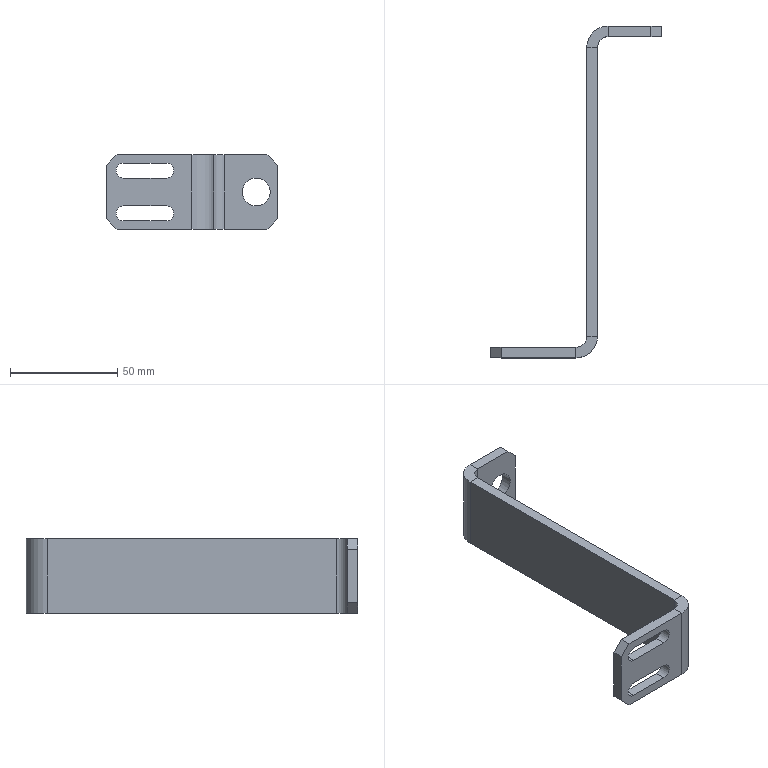Part | NX | features BREP 1 | 1 solid | 35 faces | box 80 x 155 x 35 mm | volume 36425 mm3 | plane 26 | cylinder 9 | commonest cylinder face diameters 7 x4 10 x2 20 x2 13 x1
STEP:
#1=CARTESIAN_POINT('',(0.,5.,17.5));
#2=VERTEX_POINT('',#1);
#3=CARTESIAN_POINT('',(5.,5.,17.5));
#4=VERTEX_POINT('',#3);
#5=CARTESIAN_POINT('',(0.,5.,17.5));
#6=DIRECTION('',(1.,0.,0.));
#7=VECTOR('',#6,1000.);
#8=LINE('',#5,#7);
#9=EDGE_CURVE('',#2,#4,#8,.T.);
#10=ORIENTED_EDGE('',*,*,#9,.F.);
#11=CARTESIAN_POINT('',(-5.,0.,17.5));
#12=VERTEX_POINT('',#11);
#13=CARTESIAN_POINT('',(-5.,5.,17.5));
#14=DIRECTION('',(0.,0.,1.));
#15=DIRECTION('',(-1.,0.,0.));
#16=AXIS2_PLACEMENT_3D('',#13,#14,#15);
#17=CIRCLE('',#16,5.);
#18=EDGE_CURVE('',#12,#2,#17,.T.);
#19=ORIENTED_EDGE('',*,*,#18,.F.);
#20=CARTESIAN_POINT('',(-5.,-5.,17.5));
#21=VERTEX_POINT('',#20);
#22=CARTESIAN_POINT('',(-5.,-5.,17.5));
#23=DIRECTION('',(0.,1.,0.));
#24=VECTOR('',#23,1000.);
#25=LINE('',#22,#24);
#26=EDGE_CURVE('',#21,#12,#25,.T.);
#27=ORIENTED_EDGE('',*,*,#26,.F.);
#28=CARTESIAN_POINT('',(-5.,5.,17.5));
#29=DIRECTION('',(0.,0.,1.));
#30=DIRECTION('',(1.,0.,0.));
#31=AXIS2_PLACEMENT_3D('',#28,#29,#30);
#32=CIRCLE('',#31,10.);
#33=EDGE_CURVE('',#21,#4,#32,.T.);
#34=ORIENTED_EDGE('',*,*,#33,.T.);
#35=EDGE_LOOP('',(#10,#19,#27,#34));
#36=FACE_BOUND('',#35,.T.);
#37=CARTESIAN_POINT('',(0.,5.,17.5));
#38=DIRECTION('',(0.,0.,1.));
#39=DIRECTION('',(-1.,0.,0.));
#40=AXIS2_PLACEMENT_3D('',#37,#38,#39);
#41=PLANE('',#40);
#42=ADVANCED_FACE('',(#36),#41,.T.);
#43=CARTESIAN_POINT('',(0.,140.,17.5));
#44=VERTEX_POINT('',#43);
#45=CARTESIAN_POINT('',(0.,0.,17.5));
#46=DIRECTION('',(0.,1.,0.));
#47=VECTOR('',#46,1000.);
#48=LINE('',#45,#47);
#49=EDGE_CURVE('',#2,#44,#48,.T.);
#50=ORIENTED_EDGE('',*,*,#49,.F.);
#51=ORIENTED_EDGE('',*,*,#9,.T.);
#52=CARTESIAN_POINT('',(5.,140.,17.5));
#53=VERTEX_POINT('',#52);
#54=CARTESIAN_POINT('',(5.,0.,17.5));
#55=DIRECTION('',(0.,1.,0.));
#56=VECTOR('',#55,1000.);
#57=LINE('',#54,#56);
#58=EDGE_CURVE('',#4,#53,#57,.T.);
#59=ORIENTED_EDGE('',*,*,#58,.T.);
#60=CARTESIAN_POINT('',(5.,140.,17.5));
#61=DIRECTION('',(-1.,0.,0.));
#62=VECTOR('',#61,1000.);
#63=LINE('',#60,#62);
#64=EDGE_CURVE('',#53,#44,#63,.T.);
#65=ORIENTED_EDGE('',*,*,#64,.T.);
#66=EDGE_LOOP('',(#50,#51,#59,#65));
#67=FACE_BOUND('',#66,.T.);
#68=CARTESIAN_POINT('',(-5.,-5.,17.5));
#69=DIRECTION('',(0.,0.,1.));
#70=DIRECTION('',(-1.,0.,0.));
#71=AXIS2_PLACEMENT_3D('',#68,#69,#70);
#72=PLANE('',#71);
#73=ADVANCED_FACE('',(#67),#72,.T.);
#74=CARTESIAN_POINT('',(-5.,0.,-17.5));
#75=VERTEX_POINT('',#74);
#76=CARTESIAN_POINT('',(-5.,-5.,-17.5));
#77=VERTEX_POINT('',#76);
#78=CARTESIAN_POINT('',(-5.,0.,-17.5));
#79=DIRECTION('',(0.,-1.,0.));
#80=VECTOR('',#79,1000.);
#81=LINE('',#78,#80);
#82=EDGE_CURVE('',#75,#77,#81,.T.);
#83=ORIENTED_EDGE('',*,*,#82,.F.);
#84=CARTESIAN_POINT('',(0.,5.,-17.5));
#85=VERTEX_POINT('',#84);
#86=CARTESIAN_POINT('',(-5.,5.,-17.5));
#87=DIRECTION('',(0.,0.,1.));
#88=DIRECTION('',(-1.,0.,0.));
#89=AXIS2_PLACEMENT_3D('',#86,#87,#88);
#90=CIRCLE('',#89,5.);
#91=EDGE_CURVE('',#75,#85,#90,.T.);
#92=ORIENTED_EDGE('',*,*,#91,.T.);
#93=CARTESIAN_POINT('',(5.,5.,-17.5));
#94=VERTEX_POINT('',#93);
#95=CARTESIAN_POINT('',(5.,5.,-17.5));
#96=DIRECTION('',(-1.,0.,0.));
#97=VECTOR('',#96,1000.);
#98=LINE('',#95,#97);
#99=EDGE_CURVE('',#94,#85,#98,.T.);
#100=ORIENTED_EDGE('',*,*,#99,.F.);
#101=CARTESIAN_POINT('',(-5.,5.,-17.5));
#102=DIRECTION('',(0.,0.,1.));
#103=DIRECTION('',(1.,0.,0.));
#104=AXIS2_PLACEMENT_3D('',#101,#102,#103);
#105=CIRCLE('',#104,10.);
#106=EDGE_CURVE('',#77,#94,#105,.T.);
#107=ORIENTED_EDGE('',*,*,#106,.F.);
#108=EDGE_LOOP('',(#83,#92,#100,#107));
#109=FACE_BOUND('',#108,.T.);
#110=CARTESIAN_POINT('',(-5.,0.,-17.5));
#111=DIRECTION('',(0.,0.,-1.));
#112=DIRECTION('',(1.,0.,0.));
#113=AXIS2_PLACEMENT_3D('',#110,#111,#112);
#114=PLANE('',#113);
#115=ADVANCED_FACE('',(#109),#114,.T.);
#116=CARTESIAN_POINT('',(-40.,-5.,-17.5));
#117=VERTEX_POINT('',#116);
#118=CARTESIAN_POINT('',(-45.,-5.,-17.5));
#119=DIRECTION('',(1.,0.,0.));
#120=VECTOR('',#119,1000.);
#121=LINE('',#118,#120);
#122=EDGE_CURVE('',#117,#77,#121,.T.);
#123=ORIENTED_EDGE('',*,*,#122,.F.);
#124=CARTESIAN_POINT('',(-40.,0.,-17.5));
#125=VERTEX_POINT('',#124);
#126=CARTESIAN_POINT('',(-40.,5.,-17.5));
#127=DIRECTION('',(0.,1.,0.));
#128=VECTOR('',#127,1000.);
#129=LINE('',#126,#128);
#130=EDGE_CURVE('',#117,#125,#129,.T.);
#131=ORIENTED_EDGE('',*,*,#130,.T.);
#132=CARTESIAN_POINT('',(-45.,0.,-17.5));
#133=DIRECTION('',(1.,0.,0.));
#134=VECTOR('',#133,1000.);
#135=LINE('',#132,#134);
#136=EDGE_CURVE('',#125,#75,#135,.T.);
#137=ORIENTED_EDGE('',*,*,#136,.T.);
#138=ORIENTED_EDGE('',*,*,#82,.T.);
#139=EDGE_LOOP('',(#123,#131,#137,#138));
#140=FACE_BOUND('',#139,.T.);
#141=CARTESIAN_POINT('',(5.,5.,-17.5));
#142=DIRECTION('',(0.,0.,-1.));
#143=DIRECTION('',(1.,0.,0.));
#144=AXIS2_PLACEMENT_3D('',#141,#142,#143);
#145=PLANE('',#144);
#146=ADVANCED_FACE('',(#140),#145,.T.);
#147=CARTESIAN_POINT('',(10.,150.,17.5));
#148=VERTEX_POINT('',#147);
#149=CARTESIAN_POINT('',(10.,145.,17.5));
#150=VERTEX_POINT('',#149);
#151=CARTESIAN_POINT('',(10.,150.,17.5));
#152=DIRECTION('',(0.,-1.,0.));
#153=VECTOR('',#152,1000.);
#154=LINE('',#151,#153);
#155=EDGE_CURVE('',#148,#150,#154,.T.);
#156=ORIENTED_EDGE('',*,*,#155,.F.);
#157=CARTESIAN_POINT('',(10.,140.,17.5));
#158=DIRECTION('',(0.,0.,-1.));
#159=DIRECTION('',(1.,0.,0.));
#160=AXIS2_PLACEMENT_3D('',#157,#158,#159);
#161=CIRCLE('',#160,10.);
#162=EDGE_CURVE('',#44,#148,#161,.T.);
#163=ORIENTED_EDGE('',*,*,#162,.F.);
#164=ORIENTED_EDGE('',*,*,#64,.F.);
#165=CARTESIAN_POINT('',(10.,140.,17.5));
#166=DIRECTION('',(0.,0.,-1.));
#167=DIRECTION('',(1.,0.,0.));
#168=AXIS2_PLACEMENT_3D('',#165,#166,#167);
#169=CIRCLE('',#168,5.);
#170=EDGE_CURVE('',#53,#150,#169,.T.);
#171=ORIENTED_EDGE('',*,*,#170,.T.);
#172=EDGE_LOOP('',(#156,#163,#164,#171));
#173=FACE_BOUND('',#172,.T.);
#174=CARTESIAN_POINT('',(10.,150.,17.5));
#175=DIRECTION('',(0.,0.,1.));
#176=DIRECTION('',(-1.,0.,0.));
#177=AXIS2_PLACEMENT_3D('',#174,#175,#176);
#178=PLANE('',#177);
#179=ADVANCED_FACE('',(#173),#178,.T.);
#180=CARTESIAN_POINT('',(30.,145.,17.5));
#181=VERTEX_POINT('',#180);
#182=CARTESIAN_POINT('',(0.,145.,17.5));
#183=DIRECTION('',(1.,0.,0.));
#184=VECTOR('',#183,1000.);
#185=LINE('',#182,#184);
#186=EDGE_CURVE('',#150,#181,#185,.T.);
#187=ORIENTED_EDGE('',*,*,#186,.T.);
#188=CARTESIAN_POINT('',(30.,150.,17.5));
#189=VERTEX_POINT('',#188);
#190=CARTESIAN_POINT('',(30.,140.,17.5));
#191=DIRECTION('',(0.,1.,0.));
#192=VECTOR('',#191,1000.);
#193=LINE('',#190,#192);
#194=EDGE_CURVE('',#181,#189,#193,.T.);
#195=ORIENTED_EDGE('',*,*,#194,.T.);
#196=CARTESIAN_POINT('',(0.,150.,17.5));
#197=DIRECTION('',(1.,0.,0.));
#198=VECTOR('',#197,1000.);
#199=LINE('',#196,#198);
#200=EDGE_CURVE('',#148,#189,#199,.T.);
#201=ORIENTED_EDGE('',*,*,#200,.F.);
#202=ORIENTED_EDGE('',*,*,#155,.T.);
#203=EDGE_LOOP('',(#187,#195,#201,#202));
#204=FACE_BOUND('',#203,.T.);
#205=CARTESIAN_POINT('',(5.,140.,17.5));
#206=DIRECTION('',(0.,0.,1.));
#207=DIRECTION('',(-1.,0.,0.));
#208=AXIS2_PLACEMENT_3D('',#205,#206,#207);
#209=PLANE('',#208);
#210=ADVANCED_FACE('',(#204),#209,.T.);
#211=CARTESIAN_POINT('',(0.,140.,-17.5));
#212=VERTEX_POINT('',#211);
#213=CARTESIAN_POINT('',(5.,140.,-17.5));
#214=VERTEX_POINT('',#213);
#215=CARTESIAN_POINT('',(0.,140.,-17.5));
#216=DIRECTION('',(1.,0.,0.));
#217=VECTOR('',#216,1000.);
#218=LINE('',#215,#217);
#219=EDGE_CURVE('',#212,#214,#218,.T.);
#220=ORIENTED_EDGE('',*,*,#219,.F.);
#221=CARTESIAN_POINT('',(10.,150.,-17.5));
#222=VERTEX_POINT('',#221);
#223=CARTESIAN_POINT('',(10.,140.,-17.5));
#224=DIRECTION('',(0.,0.,-1.));
#225=DIRECTION('',(1.,0.,0.));
#226=AXIS2_PLACEMENT_3D('',#223,#224,#225);
#227=CIRCLE('',#226,10.);
#228=EDGE_CURVE('',#212,#222,#227,.T.);
#229=ORIENTED_EDGE('',*,*,#228,.T.);
#230=CARTESIAN_POINT('',(10.,145.,-17.5));
#231=VERTEX_POINT('',#230);
#232=CARTESIAN_POINT('',(10.,145.,-17.5));
#233=DIRECTION('',(0.,1.,0.));
#234=VECTOR('',#233,1000.);
#235=LINE('',#232,#234);
#236=EDGE_CURVE('',#231,#222,#235,.T.);
#237=ORIENTED_EDGE('',*,*,#236,.F.);
#238=CARTESIAN_POINT('',(10.,140.,-17.5));
#239=DIRECTION('',(0.,0.,-1.));
#240=DIRECTION('',(1.,0.,0.));
#241=AXIS2_PLACEMENT_3D('',#238,#239,#240);
#242=CIRCLE('',#241,5.);
#243=EDGE_CURVE('',#214,#231,#242,.T.);
#244=ORIENTED_EDGE('',*,*,#243,.F.);
#245=EDGE_LOOP('',(#220,#229,#237,#244));
#246=FACE_BOUND('',#245,.T.);
#247=CARTESIAN_POINT('',(0.,140.,-17.5));
#248=DIRECTION('',(0.,0.,-1.));
#249=DIRECTION('',(1.,0.,0.));
#250=AXIS2_PLACEMENT_3D('',#247,#248,#249);
#251=PLANE('',#250);
#252=ADVANCED_FACE('',(#246),#251,.T.);
#253=CARTESIAN_POINT('',(0.,0.,-17.5));
#254=DIRECTION('',(0.,1.,0.));
#255=VECTOR('',#254,1000.);
#256=LINE('',#253,#255);
#257=EDGE_CURVE('',#85,#212,#256,.T.);
#258=ORIENTED_EDGE('',*,*,#257,.T.);
#259=ORIENTED_EDGE('',*,*,#219,.T.);
#260=CARTESIAN_POINT('',(5.,0.,-17.5));
#261=DIRECTION('',(0.,1.,0.));
#262=VECTOR('',#261,1000.);
#263=LINE('',#260,#262);
#264=EDGE_CURVE('',#94,#214,#263,.T.);
#265=ORIENTED_EDGE('',*,*,#264,.F.);
#266=ORIENTED_EDGE('',*,*,#99,.T.);
#267=EDGE_LOOP('',(#258,#259,#265,#266));
#268=FACE_BOUND('',#267,.T.);
#269=CARTESIAN_POINT('',(10.,145.,-17.5));
#270=DIRECTION('',(0.,0.,-1.));
#271=DIRECTION('',(1.,0.,0.));
#272=AXIS2_PLACEMENT_3D('',#269,#270,#271);
#273=PLANE('',#272);
#274=ADVANCED_FACE('',(#268),#273,.T.);
#275=CARTESIAN_POINT('',(25.,145.,6.5));
#276=VERTEX_POINT('',#275);
#277=CARTESIAN_POINT('',(25.,145.,0.));
#278=DIRECTION('',(0.,1.,0.));
#279=DIRECTION('',(0.,0.,1.));
#280=AXIS2_PLACEMENT_3D('',#277,#278,#279);
#281=CIRCLE('',#280,6.5);
#282=EDGE_CURVE('',#276,#276,#281,.T.);
#283=ORIENTED_EDGE('',*,*,#282,.T.);
#284=EDGE_LOOP('',(#283));
#285=FACE_BOUND('',#284,.T.);
#286=CARTESIAN_POINT('',(35.,145.,12.5));
#287=VERTEX_POINT('',#286);
#288=CARTESIAN_POINT('',(35.,145.,-12.5));
#289=VERTEX_POINT('',#288);
#290=CARTESIAN_POINT('',(35.,145.,17.5));
#291=DIRECTION('',(0.,0.,-1.));
#292=VECTOR('',#291,1000.);
#293=LINE('',#290,#292);
#294=EDGE_CURVE('',#287,#289,#293,.T.);
#295=ORIENTED_EDGE('',*,*,#294,.F.);
#296=CARTESIAN_POINT('',(35.,145.,12.5));
#297=DIRECTION('',(-0.7071,0.,0.7071));
#298=VECTOR('',#297,1000.);
#299=LINE('',#296,#298);
#300=EDGE_CURVE('',#287,#181,#299,.T.);
#301=ORIENTED_EDGE('',*,*,#300,.T.);
#302=ORIENTED_EDGE('',*,*,#186,.F.);
#303=CARTESIAN_POINT('',(10.,145.,17.5));
#304=DIRECTION('',(0.,0.,-1.));
#305=VECTOR('',#304,1000.);
#306=LINE('',#303,#305);
#307=EDGE_CURVE('',#150,#231,#306,.T.);
#308=ORIENTED_EDGE('',*,*,#307,.T.);
#309=CARTESIAN_POINT('',(30.,145.,-17.5));
#310=VERTEX_POINT('',#309);
#311=CARTESIAN_POINT('',(0.,145.,-17.5));
#312=DIRECTION('',(1.,0.,0.));
#313=VECTOR('',#312,1000.);
#314=LINE('',#311,#313);
#315=EDGE_CURVE('',#231,#310,#314,.T.);
#316=ORIENTED_EDGE('',*,*,#315,.T.);
#317=CARTESIAN_POINT('',(30.,145.,-17.5));
#318=DIRECTION('',(0.7071,0.,0.7071));
#319=VECTOR('',#318,1000.);
#320=LINE('',#317,#319);
#321=EDGE_CURVE('',#310,#289,#320,.T.);
#322=ORIENTED_EDGE('',*,*,#321,.T.);
#323=EDGE_LOOP('',(#295,#301,#302,#308,#316,#322));
#324=FACE_BOUND('',#323,.T.);
#325=CARTESIAN_POINT('',(0.,145.,17.5));
#326=DIRECTION('',(0.,1.,0.));
#327=DIRECTION('',(0.,0.,-1.));
#328=AXIS2_PLACEMENT_3D('',#325,#326,#327);
#329=PLANE('',#328);
#330=ADVANCED_FACE('',(#285,#324),#329,.F.);
#331=CARTESIAN_POINT('',(35.,150.,12.5));
#332=VERTEX_POINT('',#331);
#333=CARTESIAN_POINT('',(35.,150.,-12.5));
#334=VERTEX_POINT('',#333);
#335=CARTESIAN_POINT('',(35.,150.,17.5));
#336=DIRECTION('',(0.,0.,-1.));
#337=VECTOR('',#336,1000.);
#338=LINE('',#335,#337);
#339=EDGE_CURVE('',#332,#334,#338,.T.);
#340=ORIENTED_EDGE('',*,*,#339,.F.);
#341=CARTESIAN_POINT('',(35.,150.,12.5));
#342=DIRECTION('',(0.,-1.,0.));
#343=VECTOR('',#342,1000.);
#344=LINE('',#341,#343);
#345=EDGE_CURVE('',#332,#287,#344,.T.);
#346=ORIENTED_EDGE('',*,*,#345,.T.);
#347=ORIENTED_EDGE('',*,*,#294,.T.);
#348=CARTESIAN_POINT('',(35.,150.,-12.5));
#349=DIRECTION('',(0.,1.,0.));
#350=VECTOR('',#349,1000.);
#351=LINE('',#348,#350);
#352=EDGE_CURVE('',#289,#334,#351,.T.);
#353=ORIENTED_EDGE('',*,*,#352,.T.);
#354=EDGE_LOOP('',(#340,#346,#347,#353));
#355=FACE_BOUND('',#354,.T.);
#356=CARTESIAN_POINT('',(35.,150.,17.5));
#357=DIRECTION('',(1.,0.,0.));
#358=DIRECTION('',(0.,0.,1.));
#359=AXIS2_PLACEMENT_3D('',#356,#357,#358);
#360=PLANE('',#359);
#361=ADVANCED_FACE('',(#355),#360,.T.);
#362=CARTESIAN_POINT('',(25.,150.,6.5));
#363=VERTEX_POINT('',#362);
#364=CARTESIAN_POINT('',(25.,150.,0.));
#365=DIRECTION('',(0.,1.,0.));
#366=DIRECTION('',(0.,0.,1.));
#367=AXIS2_PLACEMENT_3D('',#364,#365,#366);
#368=CIRCLE('',#367,6.5);
#369=EDGE_CURVE('',#363,#363,#368,.T.);
#370=ORIENTED_EDGE('',*,*,#369,.F.);
#371=EDGE_LOOP('',(#370));
#372=FACE_BOUND('',#371,.T.);
#373=ORIENTED_EDGE('',*,*,#200,.T.);
#374=CARTESIAN_POINT('',(15.,150.,32.5));
#375=DIRECTION('',(0.7071,0.,-0.7071));
#376=VECTOR('',#375,1000.);
#377=LINE('',#374,#376);
#378=EDGE_CURVE('',#189,#332,#377,.T.);
#379=ORIENTED_EDGE('',*,*,#378,.T.);
#380=ORIENTED_EDGE('',*,*,#339,.T.);
#381=CARTESIAN_POINT('',(30.,150.,-17.5));
#382=VERTEX_POINT('',#381);
#383=CARTESIAN_POINT('',(32.5,150.,-15.));
#384=DIRECTION('',(-0.7071,0.,-0.7071));
#385=VECTOR('',#384,1000.);
#386=LINE('',#383,#385);
#387=EDGE_CURVE('',#334,#382,#386,.T.);
#388=ORIENTED_EDGE('',*,*,#387,.T.);
#389=CARTESIAN_POINT('',(0.,150.,-17.5));
#390=DIRECTION('',(1.,0.,0.));
#391=VECTOR('',#390,1000.);
#392=LINE('',#389,#391);
#393=EDGE_CURVE('',#222,#382,#392,.T.);
#394=ORIENTED_EDGE('',*,*,#393,.F.);
#395=CARTESIAN_POINT('',(10.,150.,17.5));
#396=DIRECTION('',(0.,0.,-1.));
#397=VECTOR('',#396,1000.);
#398=LINE('',#395,#397);
#399=EDGE_CURVE('',#148,#222,#398,.T.);
#400=ORIENTED_EDGE('',*,*,#399,.F.);
#401=EDGE_LOOP('',(#373,#379,#380,#388,#394,#400));
#402=FACE_BOUND('',#401,.T.);
#403=CARTESIAN_POINT('',(0.,150.,17.5));
#404=DIRECTION('',(0.,1.,0.));
#405=DIRECTION('',(0.,0.,-1.));
#406=AXIS2_PLACEMENT_3D('',#403,#404,#405);
#407=PLANE('',#406);
#408=ADVANCED_FACE('',(#372,#402),#407,.T.);
#409=ORIENTED_EDGE('',*,*,#228,.F.);
#410=CARTESIAN_POINT('',(0.,140.,17.5));
#411=DIRECTION('',(0.,0.,-1.));
#412=VECTOR('',#411,1000.);
#413=LINE('',#410,#412);
#414=EDGE_CURVE('',#44,#212,#413,.T.);
#415=ORIENTED_EDGE('',*,*,#414,.F.);
#416=ORIENTED_EDGE('',*,*,#162,.T.);
#417=ORIENTED_EDGE('',*,*,#399,.T.);
#418=EDGE_LOOP('',(#409,#415,#416,#417));
#419=FACE_BOUND('',#418,.T.);
#420=CARTESIAN_POINT('',(10.,140.,17.5));
#421=DIRECTION('',(0.,0.,-1.));
#422=DIRECTION('',(1.,0.,0.));
#423=AXIS2_PLACEMENT_3D('',#420,#421,#422);
#424=CYLINDRICAL_SURFACE('',#423,10.);
#425=ADVANCED_FACE('',(#419),#424,.T.);
#426=ORIENTED_EDGE('',*,*,#257,.F.);
#427=CARTESIAN_POINT('',(0.,5.,17.5));
#428=DIRECTION('',(0.,0.,-1.));
#429=VECTOR('',#428,1000.);
#430=LINE('',#427,#429);
#431=EDGE_CURVE('',#2,#85,#430,.T.);
#432=ORIENTED_EDGE('',*,*,#431,.F.);
#433=ORIENTED_EDGE('',*,*,#49,.T.);
#434=ORIENTED_EDGE('',*,*,#414,.T.);
#435=EDGE_LOOP('',(#426,#432,#433,#434));
#436=FACE_BOUND('',#435,.T.);
#437=CARTESIAN_POINT('',(0.,0.,17.5));
#438=DIRECTION('',(-1.,0.,0.));
#439=DIRECTION('',(0.,0.,-1.));
#440=AXIS2_PLACEMENT_3D('',#437,#438,#439);
#441=PLANE('',#440);
#442=ADVANCED_FACE('',(#436),#441,.T.);
#443=ORIENTED_EDGE('',*,*,#91,.F.);
#444=CARTESIAN_POINT('',(-5.,0.,17.5));
#445=DIRECTION('',(0.,0.,-1.));
#446=VECTOR('',#445,1000.);
#447=LINE('',#444,#446);
#448=EDGE_CURVE('',#12,#75,#447,.T.);
#449=ORIENTED_EDGE('',*,*,#448,.F.);
#450=ORIENTED_EDGE('',*,*,#18,.T.);
#451=ORIENTED_EDGE('',*,*,#431,.T.);
#452=EDGE_LOOP('',(#443,#449,#450,#451));
#453=FACE_BOUND('',#452,.T.);
#454=CARTESIAN_POINT('',(-5.,5.,17.5));
#455=DIRECTION('',(0.,0.,-1.));
#456=DIRECTION('',(1.,0.,0.));
#457=AXIS2_PLACEMENT_3D('',#454,#455,#456);
#458=CYLINDRICAL_SURFACE('',#457,5.);
#459=ADVANCED_FACE('',(#453),#458,.F.);
#460=CARTESIAN_POINT('',(-37.,0.,-13.5));
#461=VERTEX_POINT('',#460);
#462=CARTESIAN_POINT('',(-17.,0.,-13.5));
#463=VERTEX_POINT('',#462);
#464=CARTESIAN_POINT('',(-37.,0.,-13.5));
#465=DIRECTION('',(1.,0.,0.));
#466=VECTOR('',#465,1000.);
#467=LINE('',#464,#466);
#468=EDGE_CURVE('',#461,#463,#467,.T.);
#469=ORIENTED_EDGE('',*,*,#468,.T.);
#470=CARTESIAN_POINT('',(-17.,0.,-6.5));
#471=VERTEX_POINT('',#470);
#472=CARTESIAN_POINT('',(-17.,0.,-10.));
#473=DIRECTION('',(0.,-1.,0.));
#474=DIRECTION('',(0.,0.,1.));
#475=AXIS2_PLACEMENT_3D('',#472,#473,#474);
#476=CIRCLE('',#475,3.5);
#477=EDGE_CURVE('',#463,#471,#476,.T.);
#478=ORIENTED_EDGE('',*,*,#477,.T.);
#479=CARTESIAN_POINT('',(-37.,0.,-6.5));
#480=VERTEX_POINT('',#479);
#481=CARTESIAN_POINT('',(-37.,0.,-6.5));
#482=DIRECTION('',(-1.,0.,0.));
#483=VECTOR('',#482,1000.);
#484=LINE('',#481,#483);
#485=EDGE_CURVE('',#471,#480,#484,.T.);
#486=ORIENTED_EDGE('',*,*,#485,.T.);
#487=CARTESIAN_POINT('',(-37.,0.,-10.));
#488=DIRECTION('',(0.,-1.,0.));
#489=DIRECTION('',(0.,0.,1.));
#490=AXIS2_PLACEMENT_3D('',#487,#488,#489);
#491=CIRCLE('',#490,3.5);
#492=EDGE_CURVE('',#480,#461,#491,.T.);
#493=ORIENTED_EDGE('',*,*,#492,.T.);
#494=EDGE_LOOP('',(#469,#478,#486,#493));
#495=FACE_BOUND('',#494,.T.);
#496=CARTESIAN_POINT('',(-37.,0.,6.5));
#497=VERTEX_POINT('',#496);
#498=CARTESIAN_POINT('',(-17.,0.,6.5));
#499=VERTEX_POINT('',#498);
#500=CARTESIAN_POINT('',(-37.,0.,6.5));
#501=DIRECTION('',(1.,0.,0.));
#502=VECTOR('',#501,1000.);
#503=LINE('',#500,#502);
#504=EDGE_CURVE('',#497,#499,#503,.T.);
#505=ORIENTED_EDGE('',*,*,#504,.T.);
#506=CARTESIAN_POINT('',(-17.,0.,13.5));
#507=VERTEX_POINT('',#506);
#508=CARTESIAN_POINT('',(-17.,0.,10.));
#509=DIRECTION('',(0.,-1.,0.));
#510=DIRECTION('',(0.,0.,1.));
#511=AXIS2_PLACEMENT_3D('',#508,#509,#510);
#512=CIRCLE('',#511,3.5);
#513=EDGE_CURVE('',#499,#507,#512,.T.);
#514=ORIENTED_EDGE('',*,*,#513,.T.);
#515=CARTESIAN_POINT('',(-37.,0.,13.5));
#516=VERTEX_POINT('',#515);
#517=CARTESIAN_POINT('',(-37.,0.,13.5));
#518=DIRECTION('',(-1.,0.,0.));
#519=VECTOR('',#518,1000.);
#520=LINE('',#517,#519);
#521=EDGE_CURVE('',#507,#516,#520,.T.);
#522=ORIENTED_EDGE('',*,*,#521,.T.);
#523=CARTESIAN_POINT('',(-37.,0.,10.));
#524=DIRECTION('',(0.,-1.,0.));
#525=DIRECTION('',(0.,0.,1.));
#526=AXIS2_PLACEMENT_3D('',#523,#524,#525);
#527=CIRCLE('',#526,3.5);
#528=EDGE_CURVE('',#516,#497,#527,.T.);
#529=ORIENTED_EDGE('',*,*,#528,.T.);
#530=EDGE_LOOP('',(#505,#514,#522,#529));
#531=FACE_BOUND('',#530,.T.);
#532=CARTESIAN_POINT('',(-45.,0.,12.5));
#533=VERTEX_POINT('',#532);
#534=CARTESIAN_POINT('',(-45.,0.,-12.5));
#535=VERTEX_POINT('',#534);
#536=CARTESIAN_POINT('',(-45.,0.,17.5));
#537=DIRECTION('',(0.,0.,-1.));
#538=VECTOR('',#537,1000.);
#539=LINE('',#536,#538);
#540=EDGE_CURVE('',#533,#535,#539,.T.);
#541=ORIENTED_EDGE('',*,*,#540,.F.);
#542=CARTESIAN_POINT('',(-40.,0.,17.5));
#543=VERTEX_POINT('',#542);
#544=CARTESIAN_POINT('',(-42.5,0.,15.));
#545=DIRECTION('',(0.7071,0.,0.7071));
#546=VECTOR('',#545,1000.);
#547=LINE('',#544,#546);
#548=EDGE_CURVE('',#533,#543,#547,.T.);
#549=ORIENTED_EDGE('',*,*,#548,.T.);
#550=CARTESIAN_POINT('',(-45.,0.,17.5));
#551=DIRECTION('',(1.,0.,0.));
#552=VECTOR('',#551,1000.);
#553=LINE('',#550,#552);
#554=EDGE_CURVE('',#543,#12,#553,.T.);
#555=ORIENTED_EDGE('',*,*,#554,.T.);
#556=ORIENTED_EDGE('',*,*,#448,.T.);
#557=ORIENTED_EDGE('',*,*,#136,.F.);
#558=CARTESIAN_POINT('',(-60.,0.,2.5));
#559=DIRECTION('',(-0.7071,0.,0.7071));
#560=VECTOR('',#559,1000.);
#561=LINE('',#558,#560);
#562=EDGE_CURVE('',#125,#535,#561,.T.);
#563=ORIENTED_EDGE('',*,*,#562,.T.);
#564=EDGE_LOOP('',(#541,#549,#555,#556,#557,#563));
#565=FACE_BOUND('',#564,.T.);
#566=CARTESIAN_POINT('',(-45.,0.,17.5));
#567=DIRECTION('',(0.,1.,0.));
#568=DIRECTION('',(0.,0.,-1.));
#569=AXIS2_PLACEMENT_3D('',#566,#567,#568);
#570=PLANE('',#569);
#571=ADVANCED_FACE('',(#495,#531,#565),#570,.T.);
#572=CARTESIAN_POINT('',(-45.,-5.,12.5));
#573=VERTEX_POINT('',#572);
#574=CARTESIAN_POINT('',(-45.,-5.,-12.5));
#575=VERTEX_POINT('',#574);
#576=CARTESIAN_POINT('',(-45.,-5.,17.5));
#577=DIRECTION('',(0.,0.,-1.));
#578=VECTOR('',#577,1000.);
#579=LINE('',#576,#578);
#580=EDGE_CURVE('',#573,#575,#579,.T.);
#581=ORIENTED_EDGE('',*,*,#580,.F.);
#582=CARTESIAN_POINT('',(-45.,-5.,12.5));
#583=DIRECTION('',(0.,1.,0.));
#584=VECTOR('',#583,1000.);
#585=LINE('',#582,#584);
#586=EDGE_CURVE('',#573,#533,#585,.T.);
#587=ORIENTED_EDGE('',*,*,#586,.T.);
#588=ORIENTED_EDGE('',*,*,#540,.T.);
#589=CARTESIAN_POINT('',(-45.,-5.,-12.5));
#590=DIRECTION('',(0.,-1.,0.));
#591=VECTOR('',#590,1000.);
#592=LINE('',#589,#591);
#593=EDGE_CURVE('',#535,#575,#592,.T.);
#594=ORIENTED_EDGE('',*,*,#593,.T.);
#595=EDGE_LOOP('',(#581,#587,#588,#594));
#596=FACE_BOUND('',#595,.T.);
#597=CARTESIAN_POINT('',(-45.,-5.,17.5));
#598=DIRECTION('',(-1.,0.,0.));
#599=DIRECTION('',(0.,0.,-1.));
#600=AXIS2_PLACEMENT_3D('',#597,#598,#599);
#601=PLANE('',#600);
#602=ADVANCED_FACE('',(#596),#601,.T.);
#603=CARTESIAN_POINT('',(-17.,-5.,-13.5));
#604=VERTEX_POINT('',#603);
#605=CARTESIAN_POINT('',(-17.,-5.,-6.5));
#606=VERTEX_POINT('',#605);
#607=CARTESIAN_POINT('',(-17.,-5.,-10.));
#608=DIRECTION('',(0.,-1.,0.));
#609=DIRECTION('',(1.,0.,0.));
#610=AXIS2_PLACEMENT_3D('',#607,#608,#609);
#611=CIRCLE('',#610,3.5);
#612=EDGE_CURVE('',#604,#606,#611,.T.);
#613=ORIENTED_EDGE('',*,*,#612,.F.);
#614=CARTESIAN_POINT('',(-37.,-5.,-13.5));
#615=VERTEX_POINT('',#614);
#616=CARTESIAN_POINT('',(-37.,-5.,-13.5));
#617=DIRECTION('',(1.,0.,0.));
#618=VECTOR('',#617,1000.);
#619=LINE('',#616,#618);
#620=EDGE_CURVE('',#615,#604,#619,.T.);
#621=ORIENTED_EDGE('',*,*,#620,.F.);
#622=CARTESIAN_POINT('',(-37.,-5.,-6.5));
#623=VERTEX_POINT('',#622);
#624=CARTESIAN_POINT('',(-37.,-5.,-10.));
#625=DIRECTION('',(0.,-1.,0.));
#626=DIRECTION('',(1.,0.,0.));
#627=AXIS2_PLACEMENT_3D('',#624,#625,#626);
#628=CIRCLE('',#627,3.5);
#629=EDGE_CURVE('',#623,#615,#628,.T.);
#630=ORIENTED_EDGE('',*,*,#629,.F.);
#631=CARTESIAN_POINT('',(-37.,-5.,-6.5));
#632=DIRECTION('',(-1.,0.,0.));
#633=VECTOR('',#632,1000.);
#634=LINE('',#631,#633);
#635=EDGE_CURVE('',#606,#623,#634,.T.);
#636=ORIENTED_EDGE('',*,*,#635,.F.);
#637=EDGE_LOOP('',(#613,#621,#630,#636));
#638=FACE_BOUND('',#637,.T.);
#639=CARTESIAN_POINT('',(-17.,-5.,6.5));
#640=VERTEX_POINT('',#639);
#641=CARTESIAN_POINT('',(-17.,-5.,13.5));
#642=VERTEX_POINT('',#641);
#643=CARTESIAN_POINT('',(-17.,-5.,10.));
#644=DIRECTION('',(0.,-1.,0.));
#645=DIRECTION('',(1.,0.,0.));
#646=AXIS2_PLACEMENT_3D('',#643,#644,#645);
#647=CIRCLE('',#646,3.5);
#648=EDGE_CURVE('',#640,#642,#647,.T.);
#649=ORIENTED_EDGE('',*,*,#648,.F.);
#650=CARTESIAN_POINT('',(-37.,-5.,6.5));
#651=VERTEX_POINT('',#650);
#652=CARTESIAN_POINT('',(-37.,-5.,6.5));
#653=DIRECTION('',(1.,0.,0.));
#654=VECTOR('',#653,1000.);
#655=LINE('',#652,#654);
#656=EDGE_CURVE('',#651,#640,#655,.T.);
#657=ORIENTED_EDGE('',*,*,#656,.F.);
#658=CARTESIAN_POINT('',(-37.,-5.,13.5));
#659=VERTEX_POINT('',#658);
#660=CARTESIAN_POINT('',(-37.,-5.,10.));
#661=DIRECTION('',(0.,-1.,0.));
#662=DIRECTION('',(1.,0.,0.));
#663=AXIS2_PLACEMENT_3D('',#660,#661,#662);
#664=CIRCLE('',#663,3.5);
#665=EDGE_CURVE('',#659,#651,#664,.T.);
#666=ORIENTED_EDGE('',*,*,#665,.F.);
#667=CARTESIAN_POINT('',(-37.,-5.,13.5));
#668=DIRECTION('',(-1.,0.,0.));
#669=VECTOR('',#668,1000.);
#670=LINE('',#667,#669);
#671=EDGE_CURVE('',#642,#659,#670,.T.);
#672=ORIENTED_EDGE('',*,*,#671,.F.);
#673=EDGE_LOOP('',(#649,#657,#666,#672));
#674=FACE_BOUND('',#673,.T.);
#675=CARTESIAN_POINT('',(-40.,-5.,17.5));
#676=VERTEX_POINT('',#675);
#677=CARTESIAN_POINT('',(-45.,-5.,17.5));
#678=DIRECTION('',(1.,0.,0.));
#679=VECTOR('',#678,1000.);
#680=LINE('',#677,#679);
#681=EDGE_CURVE('',#676,#21,#680,.T.);
#682=ORIENTED_EDGE('',*,*,#681,.F.);
#683=CARTESIAN_POINT('',(-45.,-5.,12.5));
#684=DIRECTION('',(-0.7071,0.,-0.7071));
#685=VECTOR('',#684,1000.);
#686=LINE('',#683,#685);
#687=EDGE_CURVE('',#676,#573,#686,.T.);
#688=ORIENTED_EDGE('',*,*,#687,.T.);
#689=ORIENTED_EDGE('',*,*,#580,.T.);
#690=CARTESIAN_POINT('',(-40.,-5.,-17.5));
#691=DIRECTION('',(0.7071,0.,-0.7071));
#692=VECTOR('',#691,1000.);
#693=LINE('',#690,#692);
#694=EDGE_CURVE('',#575,#117,#693,.T.);
#695=ORIENTED_EDGE('',*,*,#694,.T.);
#696=ORIENTED_EDGE('',*,*,#122,.T.);
#697=CARTESIAN_POINT('',(-5.,-5.,17.5));
#698=DIRECTION('',(0.,0.,-1.));
#699=VECTOR('',#698,1000.);
#700=LINE('',#697,#699);
#701=EDGE_CURVE('',#21,#77,#700,.T.);
#702=ORIENTED_EDGE('',*,*,#701,.F.);
#703=EDGE_LOOP('',(#682,#688,#689,#695,#696,#702));
#704=FACE_BOUND('',#703,.T.);
#705=CARTESIAN_POINT('',(-45.,-5.,17.5));
#706=DIRECTION('',(0.,1.,0.));
#707=DIRECTION('',(0.,0.,-1.));
#708=AXIS2_PLACEMENT_3D('',#705,#706,#707);
#709=PLANE('',#708);
#710=ADVANCED_FACE('',(#638,#674,#704),#709,.F.);
#711=ORIENTED_EDGE('',*,*,#106,.T.);
#712=CARTESIAN_POINT('',(5.,5.,17.5));
#713=DIRECTION('',(0.,0.,-1.));
#714=VECTOR('',#713,1000.);
#715=LINE('',#712,#714);
#716=EDGE_CURVE('',#4,#94,#715,.T.);
#717=ORIENTED_EDGE('',*,*,#716,.F.);
#718=ORIENTED_EDGE('',*,*,#33,.F.);
#719=ORIENTED_EDGE('',*,*,#701,.T.);
#720=EDGE_LOOP('',(#711,#717,#718,#719));
#721=FACE_BOUND('',#720,.T.);
#722=CARTESIAN_POINT('',(-5.,5.,17.5));
#723=DIRECTION('',(0.,0.,-1.));
#724=DIRECTION('',(1.,0.,0.));
#725=AXIS2_PLACEMENT_3D('',#722,#723,#724);
#726=CYLINDRICAL_SURFACE('',#725,10.);
#727=ADVANCED_FACE('',(#721),#726,.T.);
#728=ORIENTED_EDGE('',*,*,#264,.T.);
#729=CARTESIAN_POINT('',(5.,140.,17.5));
#730=DIRECTION('',(0.,0.,-1.));
#731=VECTOR('',#730,1000.);
#732=LINE('',#729,#731);
#733=EDGE_CURVE('',#53,#214,#732,.T.);
#734=ORIENTED_EDGE('',*,*,#733,.F.);
#735=ORIENTED_EDGE('',*,*,#58,.F.);
#736=ORIENTED_EDGE('',*,*,#716,.T.);
#737=EDGE_LOOP('',(#728,#734,#735,#736));
#738=FACE_BOUND('',#737,.T.);
#739=CARTESIAN_POINT('',(5.,0.,17.5));
#740=DIRECTION('',(-1.,0.,0.));
#741=DIRECTION('',(0.,0.,-1.));
#742=AXIS2_PLACEMENT_3D('',#739,#740,#741);
#743=PLANE('',#742);
#744=ADVANCED_FACE('',(#738),#743,.F.);
#745=ORIENTED_EDGE('',*,*,#243,.T.);
#746=ORIENTED_EDGE('',*,*,#307,.F.);
#747=ORIENTED_EDGE('',*,*,#170,.F.);
#748=ORIENTED_EDGE('',*,*,#733,.T.);
#749=EDGE_LOOP('',(#745,#746,#747,#748));
#750=FACE_BOUND('',#749,.T.);
#751=CARTESIAN_POINT('',(10.,140.,17.5));
#752=DIRECTION('',(0.,0.,-1.));
#753=DIRECTION('',(1.,0.,0.));
#754=AXIS2_PLACEMENT_3D('',#751,#752,#753);
#755=CYLINDRICAL_SURFACE('',#754,5.);
#756=ADVANCED_FACE('',(#750),#755,.F.);
#757=ORIENTED_EDGE('',*,*,#554,.F.);
#758=CARTESIAN_POINT('',(-40.,140.,17.5));
#759=DIRECTION('',(0.,-1.,0.));
#760=VECTOR('',#759,1000.);
#761=LINE('',#758,#760);
#762=EDGE_CURVE('',#543,#676,#761,.T.);
#763=ORIENTED_EDGE('',*,*,#762,.T.);
#764=ORIENTED_EDGE('',*,*,#681,.T.);
#765=ORIENTED_EDGE('',*,*,#26,.T.);
#766=EDGE_LOOP('',(#757,#763,#764,#765));
#767=FACE_BOUND('',#766,.T.);
#768=CARTESIAN_POINT('',(10.,140.,17.5));
#769=DIRECTION('',(0.,0.,1.));
#770=DIRECTION('',(-1.,0.,0.));
#771=AXIS2_PLACEMENT_3D('',#768,#769,#770);
#772=PLANE('',#771);
#773=ADVANCED_FACE('',(#767),#772,.T.);
#774=ORIENTED_EDGE('',*,*,#393,.T.);
#775=CARTESIAN_POINT('',(30.,145.,-17.5));
#776=DIRECTION('',(0.,-1.,0.));
#777=VECTOR('',#776,1000.);
#778=LINE('',#775,#777);
#779=EDGE_CURVE('',#382,#310,#778,.T.);
#780=ORIENTED_EDGE('',*,*,#779,.T.);
#781=ORIENTED_EDGE('',*,*,#315,.F.);
#782=ORIENTED_EDGE('',*,*,#236,.T.);
#783=EDGE_LOOP('',(#774,#780,#781,#782));
#784=FACE_BOUND('',#783,.T.);
#785=CARTESIAN_POINT('',(10.,140.,-17.5));
#786=DIRECTION('',(0.,0.,1.));
#787=DIRECTION('',(-1.,0.,0.));
#788=AXIS2_PLACEMENT_3D('',#785,#786,#787);
#789=PLANE('',#788);
#790=ADVANCED_FACE('',(#784),#789,.F.);
#791=ORIENTED_EDGE('',*,*,#369,.T.);
#792=EDGE_LOOP('',(#791));
#793=FACE_BOUND('',#792,.T.);
#794=ORIENTED_EDGE('',*,*,#282,.F.);
#795=EDGE_LOOP('',(#794));
#796=FACE_BOUND('',#795,.T.);
#797=CARTESIAN_POINT('',(25.,150.,0.));
#798=DIRECTION('',(0.,1.,0.));
#799=DIRECTION('',(0.,0.,-1.));
#800=AXIS2_PLACEMENT_3D('',#797,#798,#799);
#801=CYLINDRICAL_SURFACE('',#800,6.5);
#802=ADVANCED_FACE('',(#793,#796),#801,.F.);
#803=CARTESIAN_POINT('',(-37.,27.893,6.5));
#804=DIRECTION('',(0.,-1.,0.));
#805=VECTOR('',#804,1000.);
#806=LINE('',#803,#805);
#807=EDGE_CURVE('',#497,#651,#806,.T.);
#808=ORIENTED_EDGE('',*,*,#807,.T.);
#809=ORIENTED_EDGE('',*,*,#656,.T.);
#810=CARTESIAN_POINT('',(-17.,27.893,6.5));
#811=DIRECTION('',(0.,-1.,0.));
#812=VECTOR('',#811,1000.);
#813=LINE('',#810,#812);
#814=EDGE_CURVE('',#499,#640,#813,.T.);
#815=ORIENTED_EDGE('',*,*,#814,.F.);
#816=ORIENTED_EDGE('',*,*,#504,.F.);
#817=EDGE_LOOP('',(#808,#809,#815,#816));
#818=FACE_BOUND('',#817,.T.);
#819=CARTESIAN_POINT('',(-37.,27.893,6.5));
#820=DIRECTION('',(0.,0.,-1.));
#821=DIRECTION('',(1.,0.,0.));
#822=AXIS2_PLACEMENT_3D('',#819,#820,#821);
#823=PLANE('',#822);
#824=ADVANCED_FACE('',(#818),#823,.F.);
#825=ORIENTED_EDGE('',*,*,#814,.T.);
#826=ORIENTED_EDGE('',*,*,#648,.T.);
#827=CARTESIAN_POINT('',(-17.,27.893,13.5));
#828=DIRECTION('',(0.,-1.,0.));
#829=VECTOR('',#828,1000.);
#830=LINE('',#827,#829);
#831=EDGE_CURVE('',#507,#642,#830,.T.);
#832=ORIENTED_EDGE('',*,*,#831,.F.);
#833=ORIENTED_EDGE('',*,*,#513,.F.);
#834=EDGE_LOOP('',(#825,#826,#832,#833));
#835=FACE_BOUND('',#834,.T.);
#836=CARTESIAN_POINT('',(-17.,27.893,10.));
#837=DIRECTION('',(0.,-1.,0.));
#838=DIRECTION('',(-1.,0.,0.));
#839=AXIS2_PLACEMENT_3D('',#836,#837,#838);
#840=CYLINDRICAL_SURFACE('',#839,3.5);
#841=ADVANCED_FACE('',(#835),#840,.F.);
#842=ORIENTED_EDGE('',*,*,#831,.T.);
#843=ORIENTED_EDGE('',*,*,#671,.T.);
#844=CARTESIAN_POINT('',(-37.,27.893,13.5));
#845=DIRECTION('',(0.,-1.,0.));
#846=VECTOR('',#845,1000.);
#847=LINE('',#844,#846);
#848=EDGE_CURVE('',#516,#659,#847,.T.);
#849=ORIENTED_EDGE('',*,*,#848,.F.);
#850=ORIENTED_EDGE('',*,*,#521,.F.);
#851=EDGE_LOOP('',(#842,#843,#849,#850));
#852=FACE_BOUND('',#851,.T.);
#853=CARTESIAN_POINT('',(-37.,27.893,13.5));
#854=DIRECTION('',(0.,0.,1.));
#855=DIRECTION('',(-1.,0.,0.));
#856=AXIS2_PLACEMENT_3D('',#853,#854,#855);
#857=PLANE('',#856);
#858=ADVANCED_FACE('',(#852),#857,.F.);
#859=ORIENTED_EDGE('',*,*,#848,.T.);
#860=ORIENTED_EDGE('',*,*,#665,.T.);
#861=ORIENTED_EDGE('',*,*,#807,.F.);
#862=ORIENTED_EDGE('',*,*,#528,.F.);
#863=EDGE_LOOP('',(#859,#860,#861,#862));
#864=FACE_BOUND('',#863,.T.);
#865=CARTESIAN_POINT('',(-37.,27.893,10.));
#866=DIRECTION('',(0.,-1.,0.));
#867=DIRECTION('',(-1.,0.,0.));
#868=AXIS2_PLACEMENT_3D('',#865,#866,#867);
#869=CYLINDRICAL_SURFACE('',#868,3.5);
#870=ADVANCED_FACE('',(#864),#869,.F.);
#871=CARTESIAN_POINT('',(-37.,27.893,-13.5));
#872=DIRECTION('',(0.,-1.,0.));
#873=VECTOR('',#872,1000.);
#874=LINE('',#871,#873);
#875=EDGE_CURVE('',#461,#615,#874,.T.);
#876=ORIENTED_EDGE('',*,*,#875,.T.);
#877=ORIENTED_EDGE('',*,*,#620,.T.);
#878=CARTESIAN_POINT('',(-17.,27.893,-13.5));
#879=DIRECTION('',(0.,-1.,0.));
#880=VECTOR('',#879,1000.);
#881=LINE('',#878,#880);
#882=EDGE_CURVE('',#463,#604,#881,.T.);
#883=ORIENTED_EDGE('',*,*,#882,.F.);
#884=ORIENTED_EDGE('',*,*,#468,.F.);
#885=EDGE_LOOP('',(#876,#877,#883,#884));
#886=FACE_BOUND('',#885,.T.);
#887=CARTESIAN_POINT('',(-37.,27.893,-13.5));
#888=DIRECTION('',(0.,0.,-1.));
#889=DIRECTION('',(1.,0.,0.));
#890=AXIS2_PLACEMENT_3D('',#887,#888,#889);
#891=PLANE('',#890);
#892=ADVANCED_FACE('',(#886),#891,.F.);
#893=ORIENTED_EDGE('',*,*,#882,.T.);
#894=ORIENTED_EDGE('',*,*,#612,.T.);
#895=CARTESIAN_POINT('',(-17.,27.893,-6.5));
#896=DIRECTION('',(0.,-1.,0.));
#897=VECTOR('',#896,1000.);
#898=LINE('',#895,#897);
#899=EDGE_CURVE('',#471,#606,#898,.T.);
#900=ORIENTED_EDGE('',*,*,#899,.F.);
#901=ORIENTED_EDGE('',*,*,#477,.F.);
#902=EDGE_LOOP('',(#893,#894,#900,#901));
#903=FACE_BOUND('',#902,.T.);
#904=CARTESIAN_POINT('',(-17.,27.893,-10.));
#905=DIRECTION('',(0.,-1.,0.));
#906=DIRECTION('',(-1.,0.,0.));
#907=AXIS2_PLACEMENT_3D('',#904,#905,#906);
#908=CYLINDRICAL_SURFACE('',#907,3.5);
#909=ADVANCED_FACE('',(#903),#908,.F.);
#910=ORIENTED_EDGE('',*,*,#899,.T.);
#911=ORIENTED_EDGE('',*,*,#635,.T.);
#912=CARTESIAN_POINT('',(-37.,27.893,-6.5));
#913=DIRECTION('',(0.,-1.,0.));
#914=VECTOR('',#913,1000.);
#915=LINE('',#912,#914);
#916=EDGE_CURVE('',#480,#623,#915,.T.);
#917=ORIENTED_EDGE('',*,*,#916,.F.);
#918=ORIENTED_EDGE('',*,*,#485,.F.);
#919=EDGE_LOOP('',(#910,#911,#917,#918));
#920=FACE_BOUND('',#919,.T.);
#921=CARTESIAN_POINT('',(-37.,27.893,-6.5));
#922=DIRECTION('',(0.,0.,1.));
#923=DIRECTION('',(-1.,0.,0.));
#924=AXIS2_PLACEMENT_3D('',#921,#922,#923);
#925=PLANE('',#924);
#926=ADVANCED_FACE('',(#920),#925,.F.);
#927=ORIENTED_EDGE('',*,*,#916,.T.);
#928=ORIENTED_EDGE('',*,*,#629,.T.);
#929=ORIENTED_EDGE('',*,*,#875,.F.);
#930=ORIENTED_EDGE('',*,*,#492,.F.);
#931=EDGE_LOOP('',(#927,#928,#929,#930));
#932=FACE_BOUND('',#931,.T.);
#933=CARTESIAN_POINT('',(-37.,27.893,-10.));
#934=DIRECTION('',(0.,-1.,0.));
#935=DIRECTION('',(-1.,0.,0.));
#936=AXIS2_PLACEMENT_3D('',#933,#934,#935);
#937=CYLINDRICAL_SURFACE('',#936,3.5);
#938=ADVANCED_FACE('',(#932),#937,.F.);
#939=ORIENTED_EDGE('',*,*,#378,.F.);
#940=ORIENTED_EDGE('',*,*,#194,.F.);
#941=ORIENTED_EDGE('',*,*,#300,.F.);
#942=ORIENTED_EDGE('',*,*,#345,.F.);
#943=EDGE_LOOP('',(#939,#940,#941,#942));
#944=FACE_BOUND('',#943,.T.);
#945=CARTESIAN_POINT('',(35.,150.,12.5));
#946=DIRECTION('',(-0.7071,0.,-0.7071));
#947=DIRECTION('',(0.,1.,0.));
#948=AXIS2_PLACEMENT_3D('',#945,#946,#947);
#949=PLANE('',#948);
#950=ADVANCED_FACE('',(#944),#949,.F.);
#951=ORIENTED_EDGE('',*,*,#387,.F.);
#952=ORIENTED_EDGE('',*,*,#352,.F.);
#953=ORIENTED_EDGE('',*,*,#321,.F.);
#954=ORIENTED_EDGE('',*,*,#779,.F.);
#955=EDGE_LOOP('',(#951,#952,#953,#954));
#956=FACE_BOUND('',#955,.T.);
#957=CARTESIAN_POINT('',(30.,140.,-17.5));
#958=DIRECTION('',(0.7071,0.,-0.7071));
#959=DIRECTION('',(0.,-1.,0.));
#960=AXIS2_PLACEMENT_3D('',#957,#958,#959);
#961=PLANE('',#960);
#962=ADVANCED_FACE('',(#956),#961,.T.);
#963=ORIENTED_EDGE('',*,*,#687,.F.);
#964=ORIENTED_EDGE('',*,*,#762,.F.);
#965=ORIENTED_EDGE('',*,*,#548,.F.);
#966=ORIENTED_EDGE('',*,*,#586,.F.);
#967=EDGE_LOOP('',(#963,#964,#965,#966));
#968=FACE_BOUND('',#967,.T.);
#969=CARTESIAN_POINT('',(-45.,-5.,12.5));
#970=DIRECTION('',(0.7071,0.,-0.7071));
#971=DIRECTION('',(0.,-1.,0.));
#972=AXIS2_PLACEMENT_3D('',#969,#970,#971);
#973=PLANE('',#972);
#974=ADVANCED_FACE('',(#968),#973,.F.);
#975=ORIENTED_EDGE('',*,*,#694,.F.);
#976=ORIENTED_EDGE('',*,*,#593,.F.);
#977=ORIENTED_EDGE('',*,*,#562,.F.);
#978=ORIENTED_EDGE('',*,*,#130,.F.);
#979=EDGE_LOOP('',(#975,#976,#977,#978));
#980=FACE_BOUND('',#979,.T.);
#981=CARTESIAN_POINT('',(-40.,5.,-17.5));
#982=DIRECTION('',(0.7071,0.,0.7071));
#983=DIRECTION('',(0.,-1.,0.));
#984=AXIS2_PLACEMENT_3D('',#981,#982,#983);
#985=PLANE('',#984);
#986=ADVANCED_FACE('',(#980),#985,.F.);
#987=CLOSED_SHELL('',(#42,#73,#115,#146,#179,#210,#252,#274,#330,#361,#408,#425,#442,#459,#571,#602,#710,#727,#744,#756,#773,#790,#802,#824,#841,#858,#870,#892,#909,#926,#938,#950,#962,#974,#986));
#988=MANIFOLD_SOLID_BREP('',#987);
#989=(LENGTH_UNIT()NAMED_UNIT(*)SI_UNIT(.MILLI.,.METRE.));
#990=UNCERTAINTY_MEASURE_WITH_UNIT(LENGTH_MEASURE(0.00001),#989,'','');
#991=(NAMED_UNIT(*)PLANE_ANGLE_UNIT()SI_UNIT($,.RADIAN.));
#992=(NAMED_UNIT(*)SI_UNIT($,.STERADIAN.)SOLID_ANGLE_UNIT());
#993=(GEOMETRIC_REPRESENTATION_CONTEXT(3)GLOBAL_UNCERTAINTY_ASSIGNED_CONTEXT((#990))GLOBAL_UNIT_ASSIGNED_CONTEXT((#989,#991,#992))REPRESENTATION_CONTEXT('',''));
#994=ADVANCED_BREP_SHAPE_REPRESENTATION('',(#988),#993);